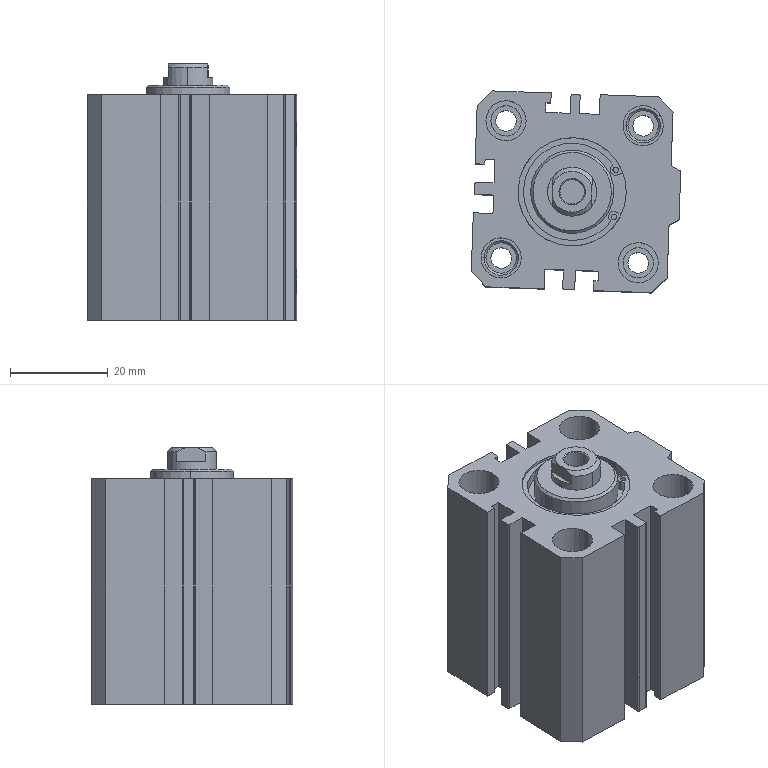Part | SolidWorks | 2 solids | 225 faces | box 42.746 x 41.177 x 52.331 mm | volume 53023 mm3 | cylinder 122 | plane 83 | cone 14 | spline 6 | commonest cylinder face diameters 5 x52 6.2 x16 8.2 x16 0.6 x8 4.2 x8 1.105 x4